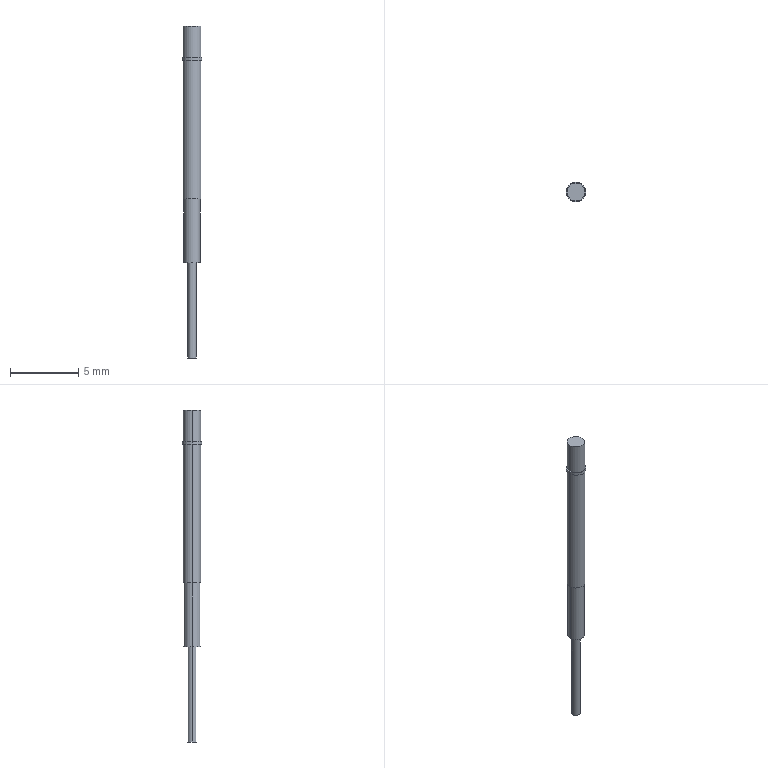Part | 1 solid | 16 faces | box 1.44 x 1.44 x 24.4 mm | volume 24.741 mm3 | cylinder 10 | plane 6 | commonest cylinder face diameters 1.31 x4 0.64 x2 1.2 x2 1.44 x2
STEP:
#1=CARTESIAN_POINT('',(1992.02,167.699,-206.5));
#2=VERTEX_POINT('',#1);
#3=CARTESIAN_POINT('',(1991.38,167.699,-206.5));
#4=VERTEX_POINT('',#3);
#5=CARTESIAN_POINT('',(1991.7,167.699,-206.5));
#6=DIRECTION('',(0.,0.,-1.));
#7=DIRECTION('',(-1.,0.,0.));
#8=AXIS2_PLACEMENT_3D('',#5,#6,#7);
#9=CIRCLE('',#8,0.32);
#10=EDGE_CURVE('',#2,#4,#9,.T.);
#11=ORIENTED_EDGE('',*,*,#10,.T.);
#12=CARTESIAN_POINT('',(1991.38,167.699,-213.5));
#13=VERTEX_POINT('',#12);
#14=CARTESIAN_POINT('',(1991.38,167.699,-213.5));
#15=DIRECTION('',(0.,0.,-1.));
#16=VECTOR('',#15,1000.);
#17=LINE('',#14,#16);
#18=EDGE_CURVE('',#13,#4,#17,.F.);
#19=ORIENTED_EDGE('',*,*,#18,.F.);
#20=CARTESIAN_POINT('',(1992.02,167.699,-213.5));
#21=VERTEX_POINT('',#20);
#22=CARTESIAN_POINT('',(1991.7,167.699,-213.5));
#23=DIRECTION('',(0.,0.,-1.));
#24=DIRECTION('',(-1.,0.,0.));
#25=AXIS2_PLACEMENT_3D('',#22,#23,#24);
#26=CIRCLE('',#25,0.32);
#27=EDGE_CURVE('',#21,#13,#26,.T.);
#28=ORIENTED_EDGE('',*,*,#27,.F.);
#29=CARTESIAN_POINT('',(1992.02,167.699,-213.5));
#30=DIRECTION('',(0.,0.,-1.));
#31=VECTOR('',#30,1000.);
#32=LINE('',#29,#31);
#33=EDGE_CURVE('',#21,#2,#32,.F.);
#34=ORIENTED_EDGE('',*,*,#33,.T.);
#35=EDGE_LOOP('',(#11,#19,#28,#34));
#36=FACE_BOUND('',#35,.T.);
#37=CARTESIAN_POINT('',(1991.7,167.699,-213.5));
#38=DIRECTION('',(0.,0.,-1.));
#39=DIRECTION('',(-1.,0.,0.));
#40=AXIS2_PLACEMENT_3D('',#37,#38,#39);
#41=CYLINDRICAL_SURFACE('',#40,0.32);
#42=ADVANCED_FACE('',(#36),#41,.T.);
#43=CARTESIAN_POINT('',(1991.1,167.699,-206.5));
#44=VERTEX_POINT('',#43);
#45=CARTESIAN_POINT('',(1992.3,167.699,-206.5));
#46=VERTEX_POINT('',#45);
#47=CARTESIAN_POINT('',(1991.7,167.699,-206.5));
#48=DIRECTION('',(0.,0.,1.));
#49=DIRECTION('',(1.,0.,0.));
#50=AXIS2_PLACEMENT_3D('',#47,#48,#49);
#51=CIRCLE('',#50,0.6);
#52=EDGE_CURVE('',#44,#46,#51,.T.);
#53=ORIENTED_EDGE('',*,*,#52,.F.);
#54=CARTESIAN_POINT('',(1991.7,167.699,-206.5));
#55=DIRECTION('',(0.,0.,1.));
#56=DIRECTION('',(1.,0.,0.));
#57=AXIS2_PLACEMENT_3D('',#54,#55,#56);
#58=CIRCLE('',#57,0.6);
#59=EDGE_CURVE('',#46,#44,#58,.T.);
#60=ORIENTED_EDGE('',*,*,#59,.F.);
#61=EDGE_LOOP('',(#53,#60));
#62=FACE_BOUND('',#61,.T.);
#63=ORIENTED_EDGE('',*,*,#10,.F.);
#64=CARTESIAN_POINT('',(1991.7,167.699,-206.5));
#65=DIRECTION('',(0.,0.,-1.));
#66=DIRECTION('',(-1.,0.,0.));
#67=AXIS2_PLACEMENT_3D('',#64,#65,#66);
#68=CIRCLE('',#67,0.32);
#69=EDGE_CURVE('',#4,#2,#68,.T.);
#70=ORIENTED_EDGE('',*,*,#69,.F.);
#71=EDGE_LOOP('',(#63,#70));
#72=FACE_BOUND('',#71,.T.);
#73=CARTESIAN_POINT('',(1991.698,167.715,-206.5));
#74=DIRECTION('',(0.,0.,1.));
#75=DIRECTION('',(1.,0.,0.));
#76=AXIS2_PLACEMENT_3D('',#73,#74,#75);
#77=PLANE('',#76);
#78=ADVANCED_FACE('',(#62,#72),#77,.F.);
#79=CARTESIAN_POINT('',(1991.1,167.699,-201.8));
#80=VERTEX_POINT('',#79);
#81=CARTESIAN_POINT('',(1992.3,167.699,-201.8));
#82=VERTEX_POINT('',#81);
#83=CARTESIAN_POINT('',(1991.7,167.699,-201.8));
#84=DIRECTION('',(0.,0.,1.));
#85=DIRECTION('',(1.,0.,0.));
#86=AXIS2_PLACEMENT_3D('',#83,#84,#85);
#87=CIRCLE('',#86,0.6);
#88=EDGE_CURVE('',#80,#82,#87,.T.);
#89=ORIENTED_EDGE('',*,*,#88,.F.);
#90=CARTESIAN_POINT('',(1991.1,167.699,-206.5));
#91=DIRECTION('',(0.,0.,1.));
#92=VECTOR('',#91,1000.);
#93=LINE('',#90,#92);
#94=EDGE_CURVE('',#44,#80,#93,.T.);
#95=ORIENTED_EDGE('',*,*,#94,.F.);
#96=ORIENTED_EDGE('',*,*,#52,.T.);
#97=CARTESIAN_POINT('',(1992.3,167.699,-206.5));
#98=DIRECTION('',(0.,0.,1.));
#99=VECTOR('',#98,1000.);
#100=LINE('',#97,#99);
#101=EDGE_CURVE('',#46,#82,#100,.T.);
#102=ORIENTED_EDGE('',*,*,#101,.T.);
#103=EDGE_LOOP('',(#89,#95,#96,#102));
#104=FACE_BOUND('',#103,.T.);
#105=CARTESIAN_POINT('',(1991.7,167.699,-206.5));
#106=DIRECTION('',(0.,0.,1.));
#107=DIRECTION('',(1.,0.,0.));
#108=AXIS2_PLACEMENT_3D('',#105,#106,#107);
#109=CYLINDRICAL_SURFACE('',#108,0.6);
#110=ADVANCED_FACE('',(#104),#109,.T.);
#111=CARTESIAN_POINT('',(1991.045,167.699,-201.8));
#112=VERTEX_POINT('',#111);
#113=CARTESIAN_POINT('',(1992.355,167.699,-201.8));
#114=VERTEX_POINT('',#113);
#115=CARTESIAN_POINT('',(1991.7,167.699,-201.8));
#116=DIRECTION('',(0.,0.,1.));
#117=DIRECTION('',(1.,0.,0.));
#118=AXIS2_PLACEMENT_3D('',#115,#116,#117);
#119=CIRCLE('',#118,0.655);
#120=EDGE_CURVE('',#112,#114,#119,.T.);
#121=ORIENTED_EDGE('',*,*,#120,.F.);
#122=CARTESIAN_POINT('',(1991.7,167.699,-201.8));
#123=DIRECTION('',(0.,0.,1.));
#124=DIRECTION('',(1.,0.,0.));
#125=AXIS2_PLACEMENT_3D('',#122,#123,#124);
#126=CIRCLE('',#125,0.655);
#127=EDGE_CURVE('',#114,#112,#126,.T.);
#128=ORIENTED_EDGE('',*,*,#127,.F.);
#129=EDGE_LOOP('',(#121,#128));
#130=FACE_BOUND('',#129,.T.);
#131=ORIENTED_EDGE('',*,*,#88,.T.);
#132=CARTESIAN_POINT('',(1991.7,167.699,-201.8));
#133=DIRECTION('',(0.,0.,1.));
#134=DIRECTION('',(1.,0.,0.));
#135=AXIS2_PLACEMENT_3D('',#132,#133,#134);
#136=CIRCLE('',#135,0.6);
#137=EDGE_CURVE('',#82,#80,#136,.T.);
#138=ORIENTED_EDGE('',*,*,#137,.T.);
#139=EDGE_LOOP('',(#131,#138));
#140=FACE_BOUND('',#139,.T.);
#141=CARTESIAN_POINT('',(1991.846,167.917,-201.8));
#142=DIRECTION('',(0.,0.,1.));
#143=DIRECTION('',(1.,0.,0.));
#144=AXIS2_PLACEMENT_3D('',#141,#142,#143);
#145=PLANE('',#144);
#146=ADVANCED_FACE('',(#130,#140),#145,.F.);
#147=CARTESIAN_POINT('',(1991.045,167.699,-191.6));
#148=VERTEX_POINT('',#147);
#149=CARTESIAN_POINT('',(1992.355,167.699,-191.6));
#150=VERTEX_POINT('',#149);
#151=CARTESIAN_POINT('',(1991.7,167.699,-191.6));
#152=DIRECTION('',(0.,0.,1.));
#153=DIRECTION('',(1.,0.,0.));
#154=AXIS2_PLACEMENT_3D('',#151,#152,#153);
#155=CIRCLE('',#154,0.655);
#156=EDGE_CURVE('',#148,#150,#155,.T.);
#157=ORIENTED_EDGE('',*,*,#156,.F.);
#158=CARTESIAN_POINT('',(1991.045,167.699,-201.8));
#159=DIRECTION('',(0.,0.,1.));
#160=VECTOR('',#159,1000.);
#161=LINE('',#158,#160);
#162=EDGE_CURVE('',#112,#148,#161,.T.);
#163=ORIENTED_EDGE('',*,*,#162,.F.);
#164=ORIENTED_EDGE('',*,*,#120,.T.);
#165=CARTESIAN_POINT('',(1992.355,167.699,-201.8));
#166=DIRECTION('',(0.,0.,1.));
#167=VECTOR('',#166,1000.);
#168=LINE('',#165,#167);
#169=EDGE_CURVE('',#114,#150,#168,.T.);
#170=ORIENTED_EDGE('',*,*,#169,.T.);
#171=EDGE_LOOP('',(#157,#163,#164,#170));
#172=FACE_BOUND('',#171,.T.);
#173=CARTESIAN_POINT('',(1991.7,167.699,-201.8));
#174=DIRECTION('',(0.,0.,1.));
#175=DIRECTION('',(1.,0.,0.));
#176=AXIS2_PLACEMENT_3D('',#173,#174,#175);
#177=CYLINDRICAL_SURFACE('',#176,0.655);
#178=ADVANCED_FACE('',(#172),#177,.T.);
#179=CARTESIAN_POINT('',(1990.98,167.699,-191.6));
#180=VERTEX_POINT('',#179);
#181=CARTESIAN_POINT('',(1992.42,167.699,-191.6));
#182=VERTEX_POINT('',#181);
#183=CARTESIAN_POINT('',(1991.7,167.699,-191.6));
#184=DIRECTION('',(0.,0.,1.));
#185=DIRECTION('',(1.,0.,0.));
#186=AXIS2_PLACEMENT_3D('',#183,#184,#185);
#187=CIRCLE('',#186,0.72);
#188=EDGE_CURVE('',#180,#182,#187,.T.);
#189=ORIENTED_EDGE('',*,*,#188,.F.);
#190=CARTESIAN_POINT('',(1991.7,167.699,-191.6));
#191=DIRECTION('',(0.,0.,1.));
#192=DIRECTION('',(1.,0.,0.));
#193=AXIS2_PLACEMENT_3D('',#190,#191,#192);
#194=CIRCLE('',#193,0.72);
#195=EDGE_CURVE('',#182,#180,#194,.T.);
#196=ORIENTED_EDGE('',*,*,#195,.F.);
#197=EDGE_LOOP('',(#189,#196));
#198=FACE_BOUND('',#197,.T.);
#199=ORIENTED_EDGE('',*,*,#156,.T.);
#200=CARTESIAN_POINT('',(1991.7,167.699,-191.6));
#201=DIRECTION('',(0.,0.,1.));
#202=DIRECTION('',(1.,0.,0.));
#203=AXIS2_PLACEMENT_3D('',#200,#201,#202);
#204=CIRCLE('',#203,0.655);
#205=EDGE_CURVE('',#150,#148,#204,.T.);
#206=ORIENTED_EDGE('',*,*,#205,.T.);
#207=EDGE_LOOP('',(#199,#206));
#208=FACE_BOUND('',#207,.T.);
#209=CARTESIAN_POINT('',(1991.69,167.646,-191.6));
#210=DIRECTION('',(0.,0.,1.));
#211=DIRECTION('',(1.,0.,0.));
#212=AXIS2_PLACEMENT_3D('',#209,#210,#211);
#213=PLANE('',#212);
#214=ADVANCED_FACE('',(#198,#208),#213,.F.);
#215=CARTESIAN_POINT('',(1990.98,167.699,-191.4));
#216=VERTEX_POINT('',#215);
#217=CARTESIAN_POINT('',(1992.42,167.699,-191.4));
#218=VERTEX_POINT('',#217);
#219=CARTESIAN_POINT('',(1991.7,167.699,-191.4));
#220=DIRECTION('',(0.,0.,1.));
#221=DIRECTION('',(1.,0.,0.));
#222=AXIS2_PLACEMENT_3D('',#219,#220,#221);
#223=CIRCLE('',#222,0.72);
#224=EDGE_CURVE('',#216,#218,#223,.T.);
#225=ORIENTED_EDGE('',*,*,#224,.F.);
#226=CARTESIAN_POINT('',(1990.98,167.699,-191.6));
#227=DIRECTION('',(0.,0.,1.));
#228=VECTOR('',#227,1000.);
#229=LINE('',#226,#228);
#230=EDGE_CURVE('',#180,#216,#229,.T.);
#231=ORIENTED_EDGE('',*,*,#230,.F.);
#232=ORIENTED_EDGE('',*,*,#188,.T.);
#233=CARTESIAN_POINT('',(1992.42,167.699,-191.6));
#234=DIRECTION('',(0.,0.,1.));
#235=VECTOR('',#234,1000.);
#236=LINE('',#233,#235);
#237=EDGE_CURVE('',#182,#218,#236,.T.);
#238=ORIENTED_EDGE('',*,*,#237,.T.);
#239=EDGE_LOOP('',(#225,#231,#232,#238));
#240=FACE_BOUND('',#239,.T.);
#241=CARTESIAN_POINT('',(1991.7,167.699,-191.6));
#242=DIRECTION('',(0.,0.,1.));
#243=DIRECTION('',(1.,0.,0.));
#244=AXIS2_PLACEMENT_3D('',#241,#242,#243);
#245=CYLINDRICAL_SURFACE('',#244,0.72);
#246=ADVANCED_FACE('',(#240),#245,.T.);
#247=ORIENTED_EDGE('',*,*,#224,.T.);
#248=CARTESIAN_POINT('',(1991.7,167.699,-191.4));
#249=DIRECTION('',(0.,0.,1.));
#250=DIRECTION('',(1.,0.,0.));
#251=AXIS2_PLACEMENT_3D('',#248,#249,#250);
#252=CIRCLE('',#251,0.72);
#253=EDGE_CURVE('',#218,#216,#252,.T.);
#254=ORIENTED_EDGE('',*,*,#253,.T.);
#255=EDGE_LOOP('',(#247,#254));
#256=FACE_BOUND('',#255,.T.);
#257=CARTESIAN_POINT('',(1991.045,167.699,-191.4));
#258=VERTEX_POINT('',#257);
#259=CARTESIAN_POINT('',(1992.355,167.699,-191.4));
#260=VERTEX_POINT('',#259);
#261=CARTESIAN_POINT('',(1991.7,167.699,-191.4));
#262=DIRECTION('',(0.,0.,1.));
#263=DIRECTION('',(1.,0.,0.));
#264=AXIS2_PLACEMENT_3D('',#261,#262,#263);
#265=CIRCLE('',#264,0.655);
#266=EDGE_CURVE('',#258,#260,#265,.T.);
#267=ORIENTED_EDGE('',*,*,#266,.F.);
#268=CARTESIAN_POINT('',(1991.7,167.699,-191.4));
#269=DIRECTION('',(0.,0.,1.));
#270=DIRECTION('',(1.,0.,0.));
#271=AXIS2_PLACEMENT_3D('',#268,#269,#270);
#272=CIRCLE('',#271,0.655);
#273=EDGE_CURVE('',#260,#258,#272,.T.);
#274=ORIENTED_EDGE('',*,*,#273,.F.);
#275=EDGE_LOOP('',(#267,#274));
#276=FACE_BOUND('',#275,.T.);
#277=CARTESIAN_POINT('',(1991.69,167.646,-191.4));
#278=DIRECTION('',(0.,0.,1.));
#279=DIRECTION('',(1.,0.,0.));
#280=AXIS2_PLACEMENT_3D('',#277,#278,#279);
#281=PLANE('',#280);
#282=ADVANCED_FACE('',(#256,#276),#281,.T.);
#283=CARTESIAN_POINT('',(1991.045,167.699,-189.1));
#284=VERTEX_POINT('',#283);
#285=CARTESIAN_POINT('',(1992.355,167.699,-189.1));
#286=VERTEX_POINT('',#285);
#287=CARTESIAN_POINT('',(1991.7,167.699,-189.1));
#288=DIRECTION('',(0.,0.,1.));
#289=DIRECTION('',(1.,0.,0.));
#290=AXIS2_PLACEMENT_3D('',#287,#288,#289);
#291=CIRCLE('',#290,0.655);
#292=EDGE_CURVE('',#284,#286,#291,.T.);
#293=ORIENTED_EDGE('',*,*,#292,.F.);
#294=CARTESIAN_POINT('',(1991.045,167.699,-191.4));
#295=DIRECTION('',(0.,0.,1.));
#296=VECTOR('',#295,1000.);
#297=LINE('',#294,#296);
#298=EDGE_CURVE('',#258,#284,#297,.T.);
#299=ORIENTED_EDGE('',*,*,#298,.F.);
#300=ORIENTED_EDGE('',*,*,#266,.T.);
#301=CARTESIAN_POINT('',(1992.355,167.699,-191.4));
#302=DIRECTION('',(0.,0.,1.));
#303=VECTOR('',#302,1000.);
#304=LINE('',#301,#303);
#305=EDGE_CURVE('',#260,#286,#304,.T.);
#306=ORIENTED_EDGE('',*,*,#305,.T.);
#307=EDGE_LOOP('',(#293,#299,#300,#306));
#308=FACE_BOUND('',#307,.T.);
#309=CARTESIAN_POINT('',(1991.7,167.699,-191.4));
#310=DIRECTION('',(0.,0.,1.));
#311=DIRECTION('',(1.,0.,0.));
#312=AXIS2_PLACEMENT_3D('',#309,#310,#311);
#313=CYLINDRICAL_SURFACE('',#312,0.655);
#314=ADVANCED_FACE('',(#308),#313,.T.);
#315=ORIENTED_EDGE('',*,*,#292,.T.);
#316=CARTESIAN_POINT('',(1991.7,167.699,-189.1));
#317=DIRECTION('',(0.,0.,1.));
#318=DIRECTION('',(1.,0.,0.));
#319=AXIS2_PLACEMENT_3D('',#316,#317,#318);
#320=CIRCLE('',#319,0.655);
#321=EDGE_CURVE('',#286,#284,#320,.T.);
#322=ORIENTED_EDGE('',*,*,#321,.T.);
#323=EDGE_LOOP('',(#315,#322));
#324=FACE_BOUND('',#323,.T.);
#325=CARTESIAN_POINT('',(1991.771,167.734,-189.1));
#326=DIRECTION('',(0.,0.,1.));
#327=DIRECTION('',(1.,0.,0.));
#328=AXIS2_PLACEMENT_3D('',#325,#326,#327);
#329=PLANE('',#328);
#330=ADVANCED_FACE('',(#324),#329,.T.);
#331=ORIENTED_EDGE('',*,*,#237,.F.);
#332=ORIENTED_EDGE('',*,*,#195,.T.);
#333=ORIENTED_EDGE('',*,*,#230,.T.);
#334=ORIENTED_EDGE('',*,*,#253,.F.);
#335=EDGE_LOOP('',(#331,#332,#333,#334));
#336=FACE_BOUND('',#335,.T.);
#337=CARTESIAN_POINT('',(1991.7,167.699,-191.6));
#338=DIRECTION('',(0.,0.,1.));
#339=DIRECTION('',(1.,0.,0.));
#340=AXIS2_PLACEMENT_3D('',#337,#338,#339);
#341=CYLINDRICAL_SURFACE('',#340,0.72);
#342=ADVANCED_FACE('',(#336),#341,.T.);
#343=ORIENTED_EDGE('',*,*,#169,.F.);
#344=ORIENTED_EDGE('',*,*,#127,.T.);
#345=ORIENTED_EDGE('',*,*,#162,.T.);
#346=ORIENTED_EDGE('',*,*,#205,.F.);
#347=EDGE_LOOP('',(#343,#344,#345,#346));
#348=FACE_BOUND('',#347,.T.);
#349=CARTESIAN_POINT('',(1991.7,167.699,-201.8));
#350=DIRECTION('',(0.,0.,1.));
#351=DIRECTION('',(1.,0.,0.));
#352=AXIS2_PLACEMENT_3D('',#349,#350,#351);
#353=CYLINDRICAL_SURFACE('',#352,0.655);
#354=ADVANCED_FACE('',(#348),#353,.T.);
#355=ORIENTED_EDGE('',*,*,#101,.F.);
#356=ORIENTED_EDGE('',*,*,#59,.T.);
#357=ORIENTED_EDGE('',*,*,#94,.T.);
#358=ORIENTED_EDGE('',*,*,#137,.F.);
#359=EDGE_LOOP('',(#355,#356,#357,#358));
#360=FACE_BOUND('',#359,.T.);
#361=CARTESIAN_POINT('',(1991.7,167.699,-206.5));
#362=DIRECTION('',(0.,0.,1.));
#363=DIRECTION('',(1.,0.,0.));
#364=AXIS2_PLACEMENT_3D('',#361,#362,#363);
#365=CYLINDRICAL_SURFACE('',#364,0.6);
#366=ADVANCED_FACE('',(#360),#365,.T.);
#367=ORIENTED_EDGE('',*,*,#305,.F.);
#368=ORIENTED_EDGE('',*,*,#273,.T.);
#369=ORIENTED_EDGE('',*,*,#298,.T.);
#370=ORIENTED_EDGE('',*,*,#321,.F.);
#371=EDGE_LOOP('',(#367,#368,#369,#370));
#372=FACE_BOUND('',#371,.T.);
#373=CARTESIAN_POINT('',(1991.7,167.699,-191.4));
#374=DIRECTION('',(0.,0.,1.));
#375=DIRECTION('',(1.,0.,0.));
#376=AXIS2_PLACEMENT_3D('',#373,#374,#375);
#377=CYLINDRICAL_SURFACE('',#376,0.655);
#378=ADVANCED_FACE('',(#372),#377,.T.);
#379=ORIENTED_EDGE('',*,*,#18,.T.);
#380=ORIENTED_EDGE('',*,*,#69,.T.);
#381=ORIENTED_EDGE('',*,*,#33,.F.);
#382=CARTESIAN_POINT('',(1991.7,167.699,-213.5));
#383=DIRECTION('',(0.,0.,-1.));
#384=DIRECTION('',(-1.,0.,0.));
#385=AXIS2_PLACEMENT_3D('',#382,#383,#384);
#386=CIRCLE('',#385,0.32);
#387=EDGE_CURVE('',#13,#21,#386,.T.);
#388=ORIENTED_EDGE('',*,*,#387,.F.);
#389=EDGE_LOOP('',(#379,#380,#381,#388));
#390=FACE_BOUND('',#389,.T.);
#391=CARTESIAN_POINT('',(1991.7,167.699,-213.5));
#392=DIRECTION('',(0.,0.,-1.));
#393=DIRECTION('',(-1.,0.,0.));
#394=AXIS2_PLACEMENT_3D('',#391,#392,#393);
#395=CYLINDRICAL_SURFACE('',#394,0.32);
#396=ADVANCED_FACE('',(#390),#395,.T.);
#397=ORIENTED_EDGE('',*,*,#27,.T.);
#398=ORIENTED_EDGE('',*,*,#387,.T.);
#399=EDGE_LOOP('',(#397,#398));
#400=FACE_BOUND('',#399,.T.);
#401=CARTESIAN_POINT('',(1985.7,138.699,-213.5));
#402=DIRECTION('',(0.,0.,-1.));
#403=DIRECTION('',(0.,-1.,0.));
#404=AXIS2_PLACEMENT_3D('',#401,#402,#403);
#405=PLANE('',#404);
#406=ADVANCED_FACE('',(#400),#405,.T.);
#407=CLOSED_SHELL('',(#42,#78,#110,#146,#178,#214,#246,#282,#314,#330,#342,#354,#366,#378,#396,#406));
#408=MANIFOLD_SOLID_BREP('',#407);
#409=(LENGTH_UNIT()NAMED_UNIT(*)SI_UNIT(.MILLI.,.METRE.));
#410=UNCERTAINTY_MEASURE_WITH_UNIT(LENGTH_MEASURE(0.00001),#409,'','');
#411=(NAMED_UNIT(*)PLANE_ANGLE_UNIT()SI_UNIT($,.RADIAN.));
#412=(NAMED_UNIT(*)SI_UNIT($,.STERADIAN.)SOLID_ANGLE_UNIT());
#413=(GEOMETRIC_REPRESENTATION_CONTEXT(3)GLOBAL_UNCERTAINTY_ASSIGNED_CONTEXT((#410))GLOBAL_UNIT_ASSIGNED_CONTEXT((#409,#411,#412))REPRESENTATION_CONTEXT('',''));
#414=ADVANCED_BREP_SHAPE_REPRESENTATION('',(#408),#413);